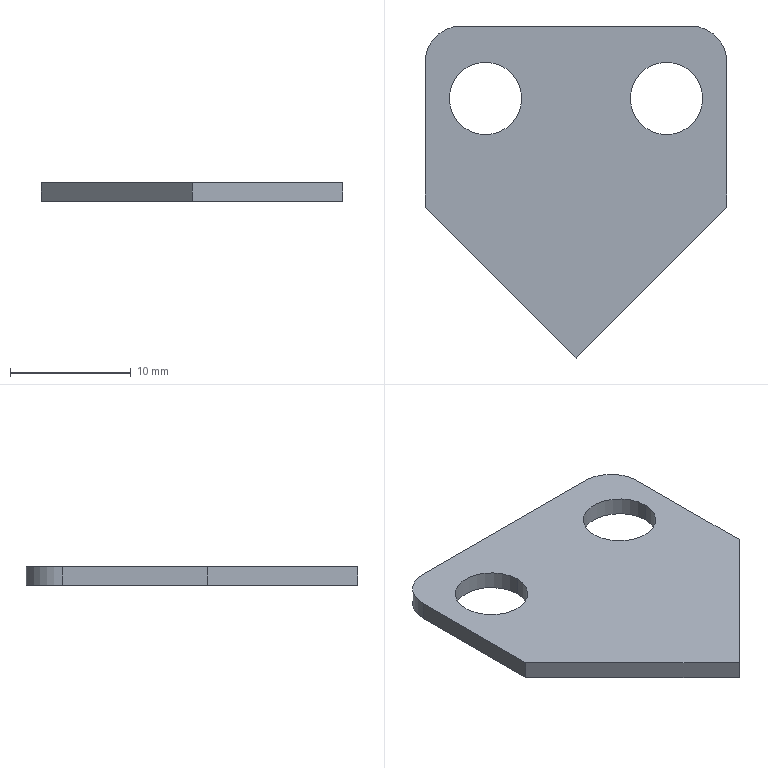Part | SolidWorks | features Extrusion 1, Fillet 1, HoleWzd 1 | 1 solid | 13 faces | box 25 x 27.5 x 1.5 mm | volume 706.258 mm3 | plane 7 | cylinder 6 | commonest cylinder face diameters 6 x6
STEP:
#1=CARTESIAN_POINT('',(-10.5,-6.,0.));
#2=VERTEX_POINT('',#1);
#3=CARTESIAN_POINT('',(-4.5,-6.,0.));
#4=VERTEX_POINT('',#3);
#5=CARTESIAN_POINT('',(-7.5,-6.,0.));
#6=DIRECTION('',(0.,0.,1.));
#7=DIRECTION('',(1.,0.,0.));
#8=AXIS2_PLACEMENT_3D('',#5,#6,#7);
#9=CIRCLE('',#8,3.);
#10=EDGE_CURVE('',#2,#4,#9,.T.);
#11=ORIENTED_EDGE('',*,*,#10,.F.);
#12=CARTESIAN_POINT('',(-10.5,-6.,1.5));
#13=VERTEX_POINT('',#12);
#14=CARTESIAN_POINT('',(-10.5,-6.,1.5));
#15=DIRECTION('',(0.,0.,1.));
#16=VECTOR('',#15,1000.);
#17=LINE('',#14,#16);
#18=EDGE_CURVE('',#2,#13,#17,.T.);
#19=ORIENTED_EDGE('',*,*,#18,.T.);
#20=CARTESIAN_POINT('',(-4.5,-6.,1.5));
#21=VERTEX_POINT('',#20);
#22=CARTESIAN_POINT('',(-7.5,-6.,1.5));
#23=DIRECTION('',(0.,0.,1.));
#24=DIRECTION('',(1.,0.,0.));
#25=AXIS2_PLACEMENT_3D('',#22,#23,#24);
#26=CIRCLE('',#25,3.);
#27=EDGE_CURVE('',#13,#21,#26,.T.);
#28=ORIENTED_EDGE('',*,*,#27,.T.);
#29=CARTESIAN_POINT('',(-4.5,-6.,1.5));
#30=DIRECTION('',(0.,0.,1.));
#31=VECTOR('',#30,1000.);
#32=LINE('',#29,#31);
#33=EDGE_CURVE('',#4,#21,#32,.T.);
#34=ORIENTED_EDGE('',*,*,#33,.F.);
#35=EDGE_LOOP('',(#11,#19,#28,#34));
#36=FACE_OUTER_BOUND('',#35,.T.);
#37=CARTESIAN_POINT('',(-7.5,-6.,1.5));
#38=DIRECTION('',(0.,0.,1.));
#39=DIRECTION('',(1.,0.,0.));
#40=AXIS2_PLACEMENT_3D('',#37,#38,#39);
#41=CYLINDRICAL_SURFACE('',#40,3.);
#42=ADVANCED_FACE('',(#36),#41,.F.);
#43=CARTESIAN_POINT('',(4.5,-6.,0.));
#44=VERTEX_POINT('',#43);
#45=CARTESIAN_POINT('',(10.5,-6.,0.));
#46=VERTEX_POINT('',#45);
#47=CARTESIAN_POINT('',(7.5,-6.,0.));
#48=DIRECTION('',(0.,0.,1.));
#49=DIRECTION('',(1.,0.,0.));
#50=AXIS2_PLACEMENT_3D('',#47,#48,#49);
#51=CIRCLE('',#50,3.);
#52=EDGE_CURVE('',#44,#46,#51,.T.);
#53=ORIENTED_EDGE('',*,*,#52,.F.);
#54=CARTESIAN_POINT('',(4.5,-6.,1.5));
#55=VERTEX_POINT('',#54);
#56=CARTESIAN_POINT('',(4.5,-6.,1.5));
#57=DIRECTION('',(0.,0.,1.));
#58=VECTOR('',#57,1000.);
#59=LINE('',#56,#58);
#60=EDGE_CURVE('',#44,#55,#59,.T.);
#61=ORIENTED_EDGE('',*,*,#60,.T.);
#62=CARTESIAN_POINT('',(10.5,-6.,1.5));
#63=VERTEX_POINT('',#62);
#64=CARTESIAN_POINT('',(7.5,-6.,1.5));
#65=DIRECTION('',(0.,0.,1.));
#66=DIRECTION('',(1.,0.,0.));
#67=AXIS2_PLACEMENT_3D('',#64,#65,#66);
#68=CIRCLE('',#67,3.);
#69=EDGE_CURVE('',#55,#63,#68,.T.);
#70=ORIENTED_EDGE('',*,*,#69,.T.);
#71=CARTESIAN_POINT('',(10.5,-6.,1.5));
#72=DIRECTION('',(0.,0.,1.));
#73=VECTOR('',#72,1000.);
#74=LINE('',#71,#73);
#75=EDGE_CURVE('',#46,#63,#74,.T.);
#76=ORIENTED_EDGE('',*,*,#75,.F.);
#77=EDGE_LOOP('',(#53,#61,#70,#76));
#78=FACE_OUTER_BOUND('',#77,.T.);
#79=CARTESIAN_POINT('',(7.5,-6.,1.5));
#80=DIRECTION('',(0.,0.,1.));
#81=DIRECTION('',(1.,0.,0.));
#82=AXIS2_PLACEMENT_3D('',#79,#80,#81);
#83=CYLINDRICAL_SURFACE('',#82,3.);
#84=ADVANCED_FACE('',(#78),#83,.F.);
#85=CARTESIAN_POINT('',(-12.5,-3.,1.5));
#86=VERTEX_POINT('',#85);
#87=CARTESIAN_POINT('',(-12.5,-15.,1.5));
#88=VERTEX_POINT('',#87);
#89=CARTESIAN_POINT('',(-12.5,-15.,1.5));
#90=DIRECTION('',(0.,-1.,0.));
#91=VECTOR('',#90,1000.);
#92=LINE('',#89,#91);
#93=EDGE_CURVE('',#86,#88,#92,.T.);
#94=ORIENTED_EDGE('',*,*,#93,.F.);
#95=CARTESIAN_POINT('',(-12.5,-3.,0.));
#96=VERTEX_POINT('',#95);
#97=CARTESIAN_POINT('',(-12.5,-3.,1.5));
#98=DIRECTION('',(0.,0.,-1.));
#99=VECTOR('',#98,1000.);
#100=LINE('',#97,#99);
#101=EDGE_CURVE('',#86,#96,#100,.T.);
#102=ORIENTED_EDGE('',*,*,#101,.T.);
#103=CARTESIAN_POINT('',(-12.5,-15.,0.));
#104=VERTEX_POINT('',#103);
#105=CARTESIAN_POINT('',(-12.5,-15.,0.));
#106=DIRECTION('',(0.,-1.,0.));
#107=VECTOR('',#106,1000.);
#108=LINE('',#105,#107);
#109=EDGE_CURVE('',#96,#104,#108,.T.);
#110=ORIENTED_EDGE('',*,*,#109,.T.);
#111=CARTESIAN_POINT('',(-12.5,-15.,1.5));
#112=DIRECTION('',(0.,0.,-1.));
#113=VECTOR('',#112,1000.);
#114=LINE('',#111,#113);
#115=EDGE_CURVE('',#88,#104,#114,.T.);
#116=ORIENTED_EDGE('',*,*,#115,.F.);
#117=EDGE_LOOP('',(#94,#102,#110,#116));
#118=FACE_OUTER_BOUND('',#117,.T.);
#119=CARTESIAN_POINT('',(-12.5,-15.,1.5));
#120=DIRECTION('',(1.,0.,0.));
#121=DIRECTION('',(0.,1.,0.));
#122=AXIS2_PLACEMENT_3D('',#119,#120,#121);
#123=PLANE('',#122);
#124=ADVANCED_FACE('',(#118),#123,.F.);
#125=CARTESIAN_POINT('',(0.,-27.5,0.));
#126=VERTEX_POINT('',#125);
#127=CARTESIAN_POINT('',(-12.5,-15.,0.));
#128=DIRECTION('',(0.7071,-0.7071,0.));
#129=VECTOR('',#128,1000.);
#130=LINE('',#127,#129);
#131=EDGE_CURVE('',#104,#126,#130,.T.);
#132=ORIENTED_EDGE('',*,*,#131,.T.);
#133=CARTESIAN_POINT('',(0.,-27.5,1.5));
#134=VERTEX_POINT('',#133);
#135=CARTESIAN_POINT('',(0.,-27.5,1.5));
#136=DIRECTION('',(0.,0.,-1.));
#137=VECTOR('',#136,1000.);
#138=LINE('',#135,#137);
#139=EDGE_CURVE('',#134,#126,#138,.T.);
#140=ORIENTED_EDGE('',*,*,#139,.F.);
#141=CARTESIAN_POINT('',(-12.5,-15.,1.5));
#142=DIRECTION('',(0.7071,-0.7071,0.));
#143=VECTOR('',#142,1000.);
#144=LINE('',#141,#143);
#145=EDGE_CURVE('',#88,#134,#144,.T.);
#146=ORIENTED_EDGE('',*,*,#145,.F.);
#147=ORIENTED_EDGE('',*,*,#115,.T.);
#148=EDGE_LOOP('',(#132,#140,#146,#147));
#149=FACE_OUTER_BOUND('',#148,.T.);
#150=CARTESIAN_POINT('',(-12.5,-15.,1.5));
#151=DIRECTION('',(0.7071,0.7071,0.));
#152=DIRECTION('',(-0.7071,0.7071,0.));
#153=AXIS2_PLACEMENT_3D('',#150,#151,#152);
#154=PLANE('',#153);
#155=ADVANCED_FACE('',(#149),#154,.F.);
#156=CARTESIAN_POINT('',(12.5,-15.,0.));
#157=VERTEX_POINT('',#156);
#158=CARTESIAN_POINT('',(0.,-27.5,0.));
#159=DIRECTION('',(0.7071,0.7071,0.));
#160=VECTOR('',#159,1000.);
#161=LINE('',#158,#160);
#162=EDGE_CURVE('',#126,#157,#161,.T.);
#163=ORIENTED_EDGE('',*,*,#162,.T.);
#164=CARTESIAN_POINT('',(12.5,-15.,1.5));
#165=VERTEX_POINT('',#164);
#166=CARTESIAN_POINT('',(12.5,-15.,1.5));
#167=DIRECTION('',(0.,0.,-1.));
#168=VECTOR('',#167,1000.);
#169=LINE('',#166,#168);
#170=EDGE_CURVE('',#165,#157,#169,.T.);
#171=ORIENTED_EDGE('',*,*,#170,.F.);
#172=CARTESIAN_POINT('',(0.,-27.5,1.5));
#173=DIRECTION('',(0.7071,0.7071,0.));
#174=VECTOR('',#173,1000.);
#175=LINE('',#172,#174);
#176=EDGE_CURVE('',#134,#165,#175,.T.);
#177=ORIENTED_EDGE('',*,*,#176,.F.);
#178=ORIENTED_EDGE('',*,*,#139,.T.);
#179=EDGE_LOOP('',(#163,#171,#177,#178));
#180=FACE_OUTER_BOUND('',#179,.T.);
#181=CARTESIAN_POINT('',(0.,-27.5,1.5));
#182=DIRECTION('',(-0.7071,0.7071,0.));
#183=DIRECTION('',(-0.7071,-0.7071,0.));
#184=AXIS2_PLACEMENT_3D('',#181,#182,#183);
#185=PLANE('',#184);
#186=ADVANCED_FACE('',(#180),#185,.F.);
#187=CARTESIAN_POINT('',(12.5,-3.,0.));
#188=VERTEX_POINT('',#187);
#189=CARTESIAN_POINT('',(12.5,0.,0.));
#190=DIRECTION('',(0.,1.,0.));
#191=VECTOR('',#190,1000.);
#192=LINE('',#189,#191);
#193=EDGE_CURVE('',#157,#188,#192,.T.);
#194=ORIENTED_EDGE('',*,*,#193,.T.);
#195=CARTESIAN_POINT('',(12.5,-3.,1.5));
#196=VERTEX_POINT('',#195);
#197=CARTESIAN_POINT('',(12.5,-3.,1.5));
#198=DIRECTION('',(0.,0.,1.));
#199=VECTOR('',#198,1000.);
#200=LINE('',#197,#199);
#201=EDGE_CURVE('',#188,#196,#200,.T.);
#202=ORIENTED_EDGE('',*,*,#201,.T.);
#203=CARTESIAN_POINT('',(12.5,0.,1.5));
#204=DIRECTION('',(0.,1.,0.));
#205=VECTOR('',#204,1000.);
#206=LINE('',#203,#205);
#207=EDGE_CURVE('',#165,#196,#206,.T.);
#208=ORIENTED_EDGE('',*,*,#207,.F.);
#209=ORIENTED_EDGE('',*,*,#170,.T.);
#210=EDGE_LOOP('',(#194,#202,#208,#209));
#211=FACE_OUTER_BOUND('',#210,.T.);
#212=CARTESIAN_POINT('',(12.5,0.,1.5));
#213=DIRECTION('',(-1.,0.,0.));
#214=DIRECTION('',(0.,-1.,0.));
#215=AXIS2_PLACEMENT_3D('',#212,#213,#214);
#216=PLANE('',#215);
#217=ADVANCED_FACE('',(#211),#216,.F.);
#218=CARTESIAN_POINT('',(9.5,0.,1.5));
#219=VERTEX_POINT('',#218);
#220=CARTESIAN_POINT('',(-9.5,0.,1.5));
#221=VERTEX_POINT('',#220);
#222=CARTESIAN_POINT('',(-12.5,0.,1.5));
#223=DIRECTION('',(-1.,0.,0.));
#224=VECTOR('',#223,1000.);
#225=LINE('',#222,#224);
#226=EDGE_CURVE('',#219,#221,#225,.T.);
#227=ORIENTED_EDGE('',*,*,#226,.F.);
#228=CARTESIAN_POINT('',(9.5,0.,0.));
#229=VERTEX_POINT('',#228);
#230=CARTESIAN_POINT('',(9.5,0.,1.5));
#231=DIRECTION('',(0.,0.,-1.));
#232=VECTOR('',#231,1000.);
#233=LINE('',#230,#232);
#234=EDGE_CURVE('',#219,#229,#233,.T.);
#235=ORIENTED_EDGE('',*,*,#234,.T.);
#236=CARTESIAN_POINT('',(-9.5,0.,0.));
#237=VERTEX_POINT('',#236);
#238=CARTESIAN_POINT('',(-12.5,0.,0.));
#239=DIRECTION('',(-1.,0.,0.));
#240=VECTOR('',#239,1000.);
#241=LINE('',#238,#240);
#242=EDGE_CURVE('',#229,#237,#241,.T.);
#243=ORIENTED_EDGE('',*,*,#242,.T.);
#244=CARTESIAN_POINT('',(-9.5,0.,1.5));
#245=DIRECTION('',(0.,0.,1.));
#246=VECTOR('',#245,1000.);
#247=LINE('',#244,#246);
#248=EDGE_CURVE('',#237,#221,#247,.T.);
#249=ORIENTED_EDGE('',*,*,#248,.T.);
#250=EDGE_LOOP('',(#227,#235,#243,#249));
#251=FACE_OUTER_BOUND('',#250,.T.);
#252=CARTESIAN_POINT('',(-12.5,0.,1.5));
#253=DIRECTION('',(0.,-1.,0.));
#254=DIRECTION('',(1.,0.,0.));
#255=AXIS2_PLACEMENT_3D('',#252,#253,#254);
#256=PLANE('',#255);
#257=ADVANCED_FACE('',(#251),#256,.F.);
#258=CARTESIAN_POINT('',(-7.5,-6.,1.5));
#259=DIRECTION('',(0.,0.,1.));
#260=DIRECTION('',(1.,0.,0.));
#261=AXIS2_PLACEMENT_3D('',#258,#259,#260);
#262=CIRCLE('',#261,3.);
#263=EDGE_CURVE('',#21,#13,#262,.T.);
#264=ORIENTED_EDGE('',*,*,#263,.F.);
#265=ORIENTED_EDGE('',*,*,#27,.F.);
#266=EDGE_LOOP('',(#264,#265));
#267=FACE_BOUND('',#266,.T.);
#268=CARTESIAN_POINT('',(7.5,-6.,1.5));
#269=DIRECTION('',(0.,0.,1.));
#270=DIRECTION('',(1.,0.,0.));
#271=AXIS2_PLACEMENT_3D('',#268,#269,#270);
#272=CIRCLE('',#271,3.);
#273=EDGE_CURVE('',#63,#55,#272,.T.);
#274=ORIENTED_EDGE('',*,*,#273,.F.);
#275=ORIENTED_EDGE('',*,*,#69,.F.);
#276=EDGE_LOOP('',(#274,#275));
#277=FACE_BOUND('',#276,.T.);
#278=ORIENTED_EDGE('',*,*,#207,.T.);
#279=CARTESIAN_POINT('',(9.5,-3.,1.5));
#280=DIRECTION('',(0.,0.,1.));
#281=DIRECTION('',(-1.,0.,0.));
#282=AXIS2_PLACEMENT_3D('',#279,#280,#281);
#283=CIRCLE('',#282,3.);
#284=EDGE_CURVE('',#196,#219,#283,.T.);
#285=ORIENTED_EDGE('',*,*,#284,.T.);
#286=ORIENTED_EDGE('',*,*,#226,.T.);
#287=CARTESIAN_POINT('',(-9.5,-3.,1.5));
#288=DIRECTION('',(0.,0.,1.));
#289=DIRECTION('',(-1.,0.,0.));
#290=AXIS2_PLACEMENT_3D('',#287,#288,#289);
#291=CIRCLE('',#290,3.);
#292=EDGE_CURVE('',#221,#86,#291,.T.);
#293=ORIENTED_EDGE('',*,*,#292,.T.);
#294=ORIENTED_EDGE('',*,*,#93,.T.);
#295=ORIENTED_EDGE('',*,*,#145,.T.);
#296=ORIENTED_EDGE('',*,*,#176,.T.);
#297=EDGE_LOOP('',(#278,#285,#286,#293,#294,#295,#296));
#298=FACE_OUTER_BOUND('',#297,.T.);
#299=CARTESIAN_POINT('',(0.,0.,1.5));
#300=DIRECTION('',(0.,0.,-1.));
#301=DIRECTION('',(-1.,0.,0.));
#302=AXIS2_PLACEMENT_3D('',#299,#300,#301);
#303=PLANE('',#302);
#304=ADVANCED_FACE('',(#267,#277,#298),#303,.F.);
#305=CARTESIAN_POINT('',(-7.5,-6.,0.));
#306=DIRECTION('',(0.,0.,1.));
#307=DIRECTION('',(1.,0.,0.));
#308=AXIS2_PLACEMENT_3D('',#305,#306,#307);
#309=CIRCLE('',#308,3.);
#310=EDGE_CURVE('',#4,#2,#309,.T.);
#311=ORIENTED_EDGE('',*,*,#310,.T.);
#312=ORIENTED_EDGE('',*,*,#10,.T.);
#313=EDGE_LOOP('',(#311,#312));
#314=FACE_BOUND('',#313,.T.);
#315=CARTESIAN_POINT('',(7.5,-6.,0.));
#316=DIRECTION('',(0.,0.,1.));
#317=DIRECTION('',(1.,0.,0.));
#318=AXIS2_PLACEMENT_3D('',#315,#316,#317);
#319=CIRCLE('',#318,3.);
#320=EDGE_CURVE('',#46,#44,#319,.T.);
#321=ORIENTED_EDGE('',*,*,#320,.T.);
#322=ORIENTED_EDGE('',*,*,#52,.T.);
#323=EDGE_LOOP('',(#321,#322));
#324=FACE_BOUND('',#323,.T.);
#325=ORIENTED_EDGE('',*,*,#242,.F.);
#326=CARTESIAN_POINT('',(9.5,-3.,0.));
#327=DIRECTION('',(0.,0.,-1.));
#328=DIRECTION('',(-1.,0.,0.));
#329=AXIS2_PLACEMENT_3D('',#326,#327,#328);
#330=CIRCLE('',#329,3.);
#331=EDGE_CURVE('',#229,#188,#330,.T.);
#332=ORIENTED_EDGE('',*,*,#331,.T.);
#333=ORIENTED_EDGE('',*,*,#193,.F.);
#334=ORIENTED_EDGE('',*,*,#162,.F.);
#335=ORIENTED_EDGE('',*,*,#131,.F.);
#336=ORIENTED_EDGE('',*,*,#109,.F.);
#337=CARTESIAN_POINT('',(-9.5,-3.,0.));
#338=DIRECTION('',(0.,0.,-1.));
#339=DIRECTION('',(-1.,0.,0.));
#340=AXIS2_PLACEMENT_3D('',#337,#338,#339);
#341=CIRCLE('',#340,3.);
#342=EDGE_CURVE('',#96,#237,#341,.T.);
#343=ORIENTED_EDGE('',*,*,#342,.T.);
#344=EDGE_LOOP('',(#325,#332,#333,#334,#335,#336,#343));
#345=FACE_OUTER_BOUND('',#344,.T.);
#346=CARTESIAN_POINT('',(0.,0.,0.));
#347=DIRECTION('',(0.,0.,-1.));
#348=DIRECTION('',(-1.,0.,0.));
#349=AXIS2_PLACEMENT_3D('',#346,#347,#348);
#350=PLANE('',#349);
#351=ADVANCED_FACE('',(#314,#324,#345),#350,.T.);
#352=ORIENTED_EDGE('',*,*,#60,.F.);
#353=ORIENTED_EDGE('',*,*,#320,.F.);
#354=ORIENTED_EDGE('',*,*,#75,.T.);
#355=ORIENTED_EDGE('',*,*,#273,.T.);
#356=EDGE_LOOP('',(#352,#353,#354,#355));
#357=FACE_OUTER_BOUND('',#356,.T.);
#358=CARTESIAN_POINT('',(7.5,-6.,1.5));
#359=DIRECTION('',(0.,0.,1.));
#360=DIRECTION('',(1.,0.,0.));
#361=AXIS2_PLACEMENT_3D('',#358,#359,#360);
#362=CYLINDRICAL_SURFACE('',#361,3.);
#363=ADVANCED_FACE('',(#357),#362,.F.);
#364=ORIENTED_EDGE('',*,*,#18,.F.);
#365=ORIENTED_EDGE('',*,*,#310,.F.);
#366=ORIENTED_EDGE('',*,*,#33,.T.);
#367=ORIENTED_EDGE('',*,*,#263,.T.);
#368=EDGE_LOOP('',(#364,#365,#366,#367));
#369=FACE_OUTER_BOUND('',#368,.T.);
#370=CARTESIAN_POINT('',(-7.5,-6.,1.5));
#371=DIRECTION('',(0.,0.,1.));
#372=DIRECTION('',(1.,0.,0.));
#373=AXIS2_PLACEMENT_3D('',#370,#371,#372);
#374=CYLINDRICAL_SURFACE('',#373,3.);
#375=ADVANCED_FACE('',(#369),#374,.F.);
#376=ORIENTED_EDGE('',*,*,#284,.F.);
#377=ORIENTED_EDGE('',*,*,#201,.F.);
#378=ORIENTED_EDGE('',*,*,#331,.F.);
#379=ORIENTED_EDGE('',*,*,#234,.F.);
#380=EDGE_LOOP('',(#376,#377,#378,#379));
#381=FACE_OUTER_BOUND('',#380,.T.);
#382=CARTESIAN_POINT('',(9.5,-3.,1.5));
#383=DIRECTION('',(0.,0.,-1.));
#384=DIRECTION('',(-1.,0.,0.));
#385=AXIS2_PLACEMENT_3D('',#382,#383,#384);
#386=CYLINDRICAL_SURFACE('',#385,3.);
#387=ADVANCED_FACE('',(#381),#386,.T.);
#388=ORIENTED_EDGE('',*,*,#292,.F.);
#389=ORIENTED_EDGE('',*,*,#248,.F.);
#390=ORIENTED_EDGE('',*,*,#342,.F.);
#391=ORIENTED_EDGE('',*,*,#101,.F.);
#392=EDGE_LOOP('',(#388,#389,#390,#391));
#393=FACE_OUTER_BOUND('',#392,.T.);
#394=CARTESIAN_POINT('',(-9.5,-3.,1.5));
#395=DIRECTION('',(0.,0.,-1.));
#396=DIRECTION('',(-1.,0.,0.));
#397=AXIS2_PLACEMENT_3D('',#394,#395,#396);
#398=CYLINDRICAL_SURFACE('',#397,3.);
#399=ADVANCED_FACE('',(#393),#398,.T.);
#400=CLOSED_SHELL('',(#42,#84,#124,#155,#186,#217,#257,#304,#351,#363,#375,#387,#399));
#401=MANIFOLD_SOLID_BREP('',#400);
#402=CARTESIAN_POINT('',(0.,0.,0.));
#403=DIRECTION('',(0.,0.,1.));
#404=DIRECTION('',(1.,0.,0.));
#405=AXIS2_PLACEMENT_3D('',#402,#403,#404);
#406=(LENGTH_UNIT()NAMED_UNIT(*)SI_UNIT(.MILLI.,.METRE.));
#407=UNCERTAINTY_MEASURE_WITH_UNIT(LENGTH_MEASURE(0.00001),#406,'','');
#408=(NAMED_UNIT(*)PLANE_ANGLE_UNIT()SI_UNIT($,.RADIAN.));
#409=(NAMED_UNIT(*)SI_UNIT($,.STERADIAN.)SOLID_ANGLE_UNIT());
#410=(GEOMETRIC_REPRESENTATION_CONTEXT(3)GLOBAL_UNCERTAINTY_ASSIGNED_CONTEXT((#407))GLOBAL_UNIT_ASSIGNED_CONTEXT((#406,#408,#409))REPRESENTATION_CONTEXT('',''));
#411=ADVANCED_BREP_SHAPE_REPRESENTATION('',(#401,#405),#410);